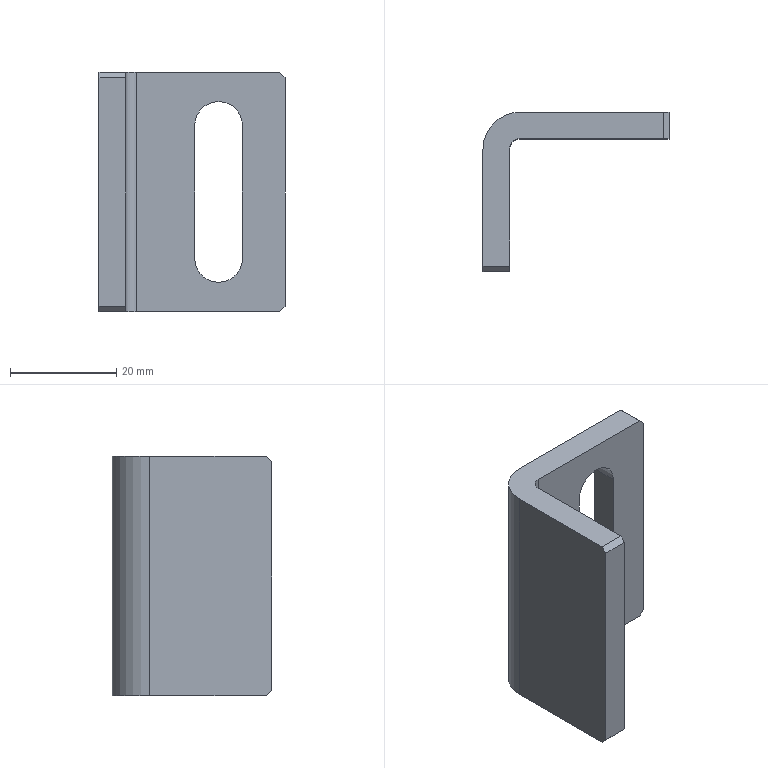Part | SolidWorks | features Fillet 2, Chamfer 1, ExtruThin 1, ICE 1 | 1 solid | 19 faces | box 35 x 30 x 45 mm | volume 11612 mm3 | plane 14 | cylinder 5 | commonest cylinder face diameters 9 x3 4 x1 14 x1
STEP:
#1=CARTESIAN_POINT('',(22.5,30.,5.5));
#2=VERTEX_POINT('',#1);
#3=CARTESIAN_POINT('',(27.,30.,10.));
#4=VERTEX_POINT('',#3);
#5=CARTESIAN_POINT('',(22.5,30.,10.));
#6=DIRECTION('',(0.,-1.,0.));
#7=DIRECTION('',(0.,0.,-1.));
#8=AXIS2_PLACEMENT_3D('',#5,#6,#7);
#9=CIRCLE('',#8,4.5);
#10=EDGE_CURVE('',#2,#4,#9,.T.);
#11=ORIENTED_EDGE('',*,*,#10,.F.);
#12=CARTESIAN_POINT('',(22.5,25.,5.5));
#13=VERTEX_POINT('',#12);
#14=CARTESIAN_POINT('',(22.5,30.,5.5));
#15=DIRECTION('',(0.,-1.,0.));
#16=VECTOR('',#15,1000.);
#17=LINE('',#14,#16);
#18=EDGE_CURVE('',#2,#13,#17,.T.);
#19=ORIENTED_EDGE('',*,*,#18,.T.);
#20=CARTESIAN_POINT('',(27.,25.,10.));
#21=VERTEX_POINT('',#20);
#22=CARTESIAN_POINT('',(22.5,25.,10.));
#23=DIRECTION('',(0.,-1.,0.));
#24=DIRECTION('',(0.,0.,-1.));
#25=AXIS2_PLACEMENT_3D('',#22,#23,#24);
#26=CIRCLE('',#25,4.5);
#27=EDGE_CURVE('',#13,#21,#26,.T.);
#28=ORIENTED_EDGE('',*,*,#27,.T.);
#29=CARTESIAN_POINT('',(27.,30.,10.));
#30=DIRECTION('',(0.,-1.,0.));
#31=VECTOR('',#30,1000.);
#32=LINE('',#29,#31);
#33=EDGE_CURVE('',#4,#21,#32,.T.);
#34=ORIENTED_EDGE('',*,*,#33,.F.);
#35=EDGE_LOOP('',(#11,#19,#28,#34));
#36=FACE_OUTER_BOUND('',#35,.T.);
#37=CARTESIAN_POINT('',(22.5,30.,10.));
#38=DIRECTION('',(0.,-1.,0.));
#39=DIRECTION('',(0.,0.,-1.));
#40=AXIS2_PLACEMENT_3D('',#37,#38,#39);
#41=CYLINDRICAL_SURFACE('',#40,4.5);
#42=ADVANCED_FACE('',(#36),#41,.F.);
#43=CARTESIAN_POINT('',(18.,25.,35.));
#44=VERTEX_POINT('',#43);
#45=CARTESIAN_POINT('',(18.,25.,10.));
#46=VERTEX_POINT('',#45);
#47=CARTESIAN_POINT('',(18.,25.,35.));
#48=DIRECTION('',(0.,0.,-1.));
#49=VECTOR('',#48,1000.);
#50=LINE('',#47,#49);
#51=EDGE_CURVE('',#44,#46,#50,.T.);
#52=ORIENTED_EDGE('',*,*,#51,.F.);
#53=CARTESIAN_POINT('',(27.,25.,35.));
#54=VERTEX_POINT('',#53);
#55=CARTESIAN_POINT('',(22.5,25.,35.));
#56=DIRECTION('',(0.,-1.,0.));
#57=DIRECTION('',(0.,0.,-1.));
#58=AXIS2_PLACEMENT_3D('',#55,#56,#57);
#59=CIRCLE('',#58,4.5);
#60=EDGE_CURVE('',#54,#44,#59,.T.);
#61=ORIENTED_EDGE('',*,*,#60,.F.);
#62=CARTESIAN_POINT('',(27.,25.,35.));
#63=DIRECTION('',(0.,0.,1.));
#64=VECTOR('',#63,1000.);
#65=LINE('',#62,#64);
#66=EDGE_CURVE('',#21,#54,#65,.T.);
#67=ORIENTED_EDGE('',*,*,#66,.F.);
#68=ORIENTED_EDGE('',*,*,#27,.F.);
#69=CARTESIAN_POINT('',(22.5,25.,10.));
#70=DIRECTION('',(0.,-1.,0.));
#71=DIRECTION('',(0.,0.,-1.));
#72=AXIS2_PLACEMENT_3D('',#69,#70,#71);
#73=CIRCLE('',#72,4.5);
#74=EDGE_CURVE('',#46,#13,#73,.T.);
#75=ORIENTED_EDGE('',*,*,#74,.F.);
#76=EDGE_LOOP('',(#52,#61,#67,#68,#75));
#77=FACE_BOUND('',#76,.T.);
#78=CARTESIAN_POINT('',(7.,25.,0.));
#79=VERTEX_POINT('',#78);
#80=CARTESIAN_POINT('',(34.,25.,0.));
#81=VERTEX_POINT('',#80);
#82=CARTESIAN_POINT('',(0.,25.,0.));
#83=DIRECTION('',(1.,0.,0.));
#84=VECTOR('',#83,1000.);
#85=LINE('',#82,#84);
#86=EDGE_CURVE('',#79,#81,#85,.T.);
#87=ORIENTED_EDGE('',*,*,#86,.T.);
#88=CARTESIAN_POINT('',(35.,25.,1.));
#89=VERTEX_POINT('',#88);
#90=CARTESIAN_POINT('',(34.,25.,0.));
#91=DIRECTION('',(0.7071,0.,0.7071));
#92=VECTOR('',#91,1000.);
#93=LINE('',#90,#92);
#94=EDGE_CURVE('',#81,#89,#93,.T.);
#95=ORIENTED_EDGE('',*,*,#94,.T.);
#96=CARTESIAN_POINT('',(35.,25.,44.));
#97=VERTEX_POINT('',#96);
#98=CARTESIAN_POINT('',(35.,25.,45.));
#99=DIRECTION('',(0.,0.,-1.));
#100=VECTOR('',#99,1000.);
#101=LINE('',#98,#100);
#102=EDGE_CURVE('',#97,#89,#101,.T.);
#103=ORIENTED_EDGE('',*,*,#102,.F.);
#104=CARTESIAN_POINT('',(34.,25.,45.));
#105=VERTEX_POINT('',#104);
#106=CARTESIAN_POINT('',(35.,25.,44.));
#107=DIRECTION('',(-0.7071,0.,0.7071));
#108=VECTOR('',#107,1000.);
#109=LINE('',#106,#108);
#110=EDGE_CURVE('',#97,#105,#109,.T.);
#111=ORIENTED_EDGE('',*,*,#110,.T.);
#112=CARTESIAN_POINT('',(7.,25.,45.));
#113=VERTEX_POINT('',#112);
#114=CARTESIAN_POINT('',(0.,25.,45.));
#115=DIRECTION('',(1.,0.,0.));
#116=VECTOR('',#115,1000.);
#117=LINE('',#114,#116);
#118=EDGE_CURVE('',#113,#105,#117,.T.);
#119=ORIENTED_EDGE('',*,*,#118,.F.);
#120=CARTESIAN_POINT('',(7.,25.,0.));
#121=DIRECTION('',(0.,0.,-1.));
#122=VECTOR('',#121,1000.);
#123=LINE('',#120,#122);
#124=EDGE_CURVE('',#113,#79,#123,.T.);
#125=ORIENTED_EDGE('',*,*,#124,.T.);
#126=EDGE_LOOP('',(#87,#95,#103,#111,#119,#125));
#127=FACE_OUTER_BOUND('',#126,.T.);
#128=CARTESIAN_POINT('',(0.,25.,45.));
#129=DIRECTION('',(0.,1.,0.));
#130=DIRECTION('',(0.,0.,1.));
#131=AXIS2_PLACEMENT_3D('',#128,#129,#130);
#132=PLANE('',#131);
#133=ADVANCED_FACE('',(#77,#127),#132,.F.);
#134=ORIENTED_EDGE('',*,*,#102,.T.);
#135=CARTESIAN_POINT('',(35.,30.,1.));
#136=VERTEX_POINT('',#135);
#137=CARTESIAN_POINT('',(35.,30.,1.));
#138=DIRECTION('',(0.,1.,0.));
#139=VECTOR('',#138,1000.);
#140=LINE('',#137,#139);
#141=EDGE_CURVE('',#89,#136,#140,.T.);
#142=ORIENTED_EDGE('',*,*,#141,.T.);
#143=CARTESIAN_POINT('',(35.,30.,44.));
#144=VERTEX_POINT('',#143);
#145=CARTESIAN_POINT('',(35.,30.,45.));
#146=DIRECTION('',(0.,0.,-1.));
#147=VECTOR('',#146,1000.);
#148=LINE('',#145,#147);
#149=EDGE_CURVE('',#144,#136,#148,.T.);
#150=ORIENTED_EDGE('',*,*,#149,.F.);
#151=CARTESIAN_POINT('',(35.,25.,44.));
#152=DIRECTION('',(0.,-1.,0.));
#153=VECTOR('',#152,1000.);
#154=LINE('',#151,#153);
#155=EDGE_CURVE('',#144,#97,#154,.T.);
#156=ORIENTED_EDGE('',*,*,#155,.T.);
#157=EDGE_LOOP('',(#134,#142,#150,#156));
#158=FACE_OUTER_BOUND('',#157,.T.);
#159=CARTESIAN_POINT('',(35.,30.,45.));
#160=DIRECTION('',(1.,0.,0.));
#161=DIRECTION('',(0.,0.,-1.));
#162=AXIS2_PLACEMENT_3D('',#159,#160,#161);
#163=PLANE('',#162);
#164=ADVANCED_FACE('',(#158),#163,.T.);
#165=CARTESIAN_POINT('',(27.,30.,35.));
#166=VERTEX_POINT('',#165);
#167=CARTESIAN_POINT('',(18.,30.,35.));
#168=VERTEX_POINT('',#167);
#169=CARTESIAN_POINT('',(22.5,30.,35.));
#170=DIRECTION('',(0.,-1.,0.));
#171=DIRECTION('',(0.,0.,-1.));
#172=AXIS2_PLACEMENT_3D('',#169,#170,#171);
#173=CIRCLE('',#172,4.5);
#174=EDGE_CURVE('',#166,#168,#173,.T.);
#175=ORIENTED_EDGE('',*,*,#174,.T.);
#176=CARTESIAN_POINT('',(18.,30.,10.));
#177=VERTEX_POINT('',#176);
#178=CARTESIAN_POINT('',(18.,30.,35.));
#179=DIRECTION('',(0.,0.,-1.));
#180=VECTOR('',#179,1000.);
#181=LINE('',#178,#180);
#182=EDGE_CURVE('',#168,#177,#181,.T.);
#183=ORIENTED_EDGE('',*,*,#182,.T.);
#184=CARTESIAN_POINT('',(22.5,30.,10.));
#185=DIRECTION('',(0.,-1.,0.));
#186=DIRECTION('',(0.,0.,-1.));
#187=AXIS2_PLACEMENT_3D('',#184,#185,#186);
#188=CIRCLE('',#187,4.5);
#189=EDGE_CURVE('',#177,#2,#188,.T.);
#190=ORIENTED_EDGE('',*,*,#189,.T.);
#191=ORIENTED_EDGE('',*,*,#10,.T.);
#192=CARTESIAN_POINT('',(27.,30.,35.));
#193=DIRECTION('',(0.,0.,1.));
#194=VECTOR('',#193,1000.);
#195=LINE('',#192,#194);
#196=EDGE_CURVE('',#4,#166,#195,.T.);
#197=ORIENTED_EDGE('',*,*,#196,.T.);
#198=EDGE_LOOP('',(#175,#183,#190,#191,#197));
#199=FACE_BOUND('',#198,.T.);
#200=ORIENTED_EDGE('',*,*,#149,.T.);
#201=CARTESIAN_POINT('',(34.,30.,0.));
#202=VERTEX_POINT('',#201);
#203=CARTESIAN_POINT('',(39.5,30.,5.5));
#204=DIRECTION('',(-0.7071,0.,-0.7071));
#205=VECTOR('',#204,1000.);
#206=LINE('',#203,#205);
#207=EDGE_CURVE('',#136,#202,#206,.T.);
#208=ORIENTED_EDGE('',*,*,#207,.T.);
#209=CARTESIAN_POINT('',(7.,30.,0.));
#210=VERTEX_POINT('',#209);
#211=CARTESIAN_POINT('',(0.,30.,0.));
#212=DIRECTION('',(1.,0.,0.));
#213=VECTOR('',#212,1000.);
#214=LINE('',#211,#213);
#215=EDGE_CURVE('',#210,#202,#214,.T.);
#216=ORIENTED_EDGE('',*,*,#215,.F.);
#217=CARTESIAN_POINT('',(7.,30.,45.));
#218=VERTEX_POINT('',#217);
#219=CARTESIAN_POINT('',(7.,30.,45.));
#220=DIRECTION('',(0.,0.,1.));
#221=VECTOR('',#220,1000.);
#222=LINE('',#219,#221);
#223=EDGE_CURVE('',#210,#218,#222,.T.);
#224=ORIENTED_EDGE('',*,*,#223,.T.);
#225=CARTESIAN_POINT('',(34.,30.,45.));
#226=VERTEX_POINT('',#225);
#227=CARTESIAN_POINT('',(0.,30.,45.));
#228=DIRECTION('',(1.,0.,0.));
#229=VECTOR('',#228,1000.);
#230=LINE('',#227,#229);
#231=EDGE_CURVE('',#218,#226,#230,.T.);
#232=ORIENTED_EDGE('',*,*,#231,.T.);
#233=CARTESIAN_POINT('',(17.,30.,62.));
#234=DIRECTION('',(0.7071,0.,-0.7071));
#235=VECTOR('',#234,1000.);
#236=LINE('',#233,#235);
#237=EDGE_CURVE('',#226,#144,#236,.T.);
#238=ORIENTED_EDGE('',*,*,#237,.T.);
#239=EDGE_LOOP('',(#200,#208,#216,#224,#232,#238));
#240=FACE_OUTER_BOUND('',#239,.T.);
#241=CARTESIAN_POINT('',(0.,30.,45.));
#242=DIRECTION('',(0.,1.,0.));
#243=DIRECTION('',(0.,0.,1.));
#244=AXIS2_PLACEMENT_3D('',#241,#242,#243);
#245=PLANE('',#244);
#246=ADVANCED_FACE('',(#199,#240),#245,.T.);
#247=CARTESIAN_POINT('',(0.,1.,0.));
#248=VERTEX_POINT('',#247);
#249=CARTESIAN_POINT('',(0.,23.,0.));
#250=VERTEX_POINT('',#249);
#251=CARTESIAN_POINT('',(0.,0.,0.));
#252=DIRECTION('',(0.,1.,0.));
#253=VECTOR('',#252,1000.);
#254=LINE('',#251,#253);
#255=EDGE_CURVE('',#248,#250,#254,.T.);
#256=ORIENTED_EDGE('',*,*,#255,.F.);
#257=CARTESIAN_POINT('',(0.,0.,1.));
#258=VERTEX_POINT('',#257);
#259=CARTESIAN_POINT('',(0.,-22.,23.));
#260=DIRECTION('',(0.,-0.7071,0.7071));
#261=VECTOR('',#260,1000.);
#262=LINE('',#259,#261);
#263=EDGE_CURVE('',#248,#258,#262,.T.);
#264=ORIENTED_EDGE('',*,*,#263,.T.);
#265=CARTESIAN_POINT('',(0.,0.,44.));
#266=VERTEX_POINT('',#265);
#267=CARTESIAN_POINT('',(0.,0.,45.));
#268=DIRECTION('',(0.,0.,-1.));
#269=VECTOR('',#268,1000.);
#270=LINE('',#267,#269);
#271=EDGE_CURVE('',#266,#258,#270,.T.);
#272=ORIENTED_EDGE('',*,*,#271,.F.);
#273=CARTESIAN_POINT('',(0.,1.,45.));
#274=VERTEX_POINT('',#273);
#275=CARTESIAN_POINT('',(0.,0.5,44.5));
#276=DIRECTION('',(0.,0.7071,0.7071));
#277=VECTOR('',#276,1000.);
#278=LINE('',#275,#277);
#279=EDGE_CURVE('',#266,#274,#278,.T.);
#280=ORIENTED_EDGE('',*,*,#279,.T.);
#281=CARTESIAN_POINT('',(0.,23.,45.));
#282=VERTEX_POINT('',#281);
#283=CARTESIAN_POINT('',(0.,0.,45.));
#284=DIRECTION('',(0.,1.,0.));
#285=VECTOR('',#284,1000.);
#286=LINE('',#283,#285);
#287=EDGE_CURVE('',#274,#282,#286,.T.);
#288=ORIENTED_EDGE('',*,*,#287,.T.);
#289=CARTESIAN_POINT('',(0.,23.,45.));
#290=DIRECTION('',(0.,0.,-1.));
#291=VECTOR('',#290,1000.);
#292=LINE('',#289,#291);
#293=EDGE_CURVE('',#282,#250,#292,.T.);
#294=ORIENTED_EDGE('',*,*,#293,.T.);
#295=EDGE_LOOP('',(#256,#264,#272,#280,#288,#294));
#296=FACE_OUTER_BOUND('',#295,.T.);
#297=CARTESIAN_POINT('',(0.,0.,45.));
#298=DIRECTION('',(-1.,0.,0.));
#299=DIRECTION('',(0.,0.,1.));
#300=AXIS2_PLACEMENT_3D('',#297,#298,#299);
#301=PLANE('',#300);
#302=ADVANCED_FACE('',(#296),#301,.T.);
#303=ORIENTED_EDGE('',*,*,#271,.T.);
#304=CARTESIAN_POINT('',(5.,0.,1.));
#305=VERTEX_POINT('',#304);
#306=CARTESIAN_POINT('',(5.,0.,1.));
#307=DIRECTION('',(1.,0.,0.));
#308=VECTOR('',#307,1000.);
#309=LINE('',#306,#308);
#310=EDGE_CURVE('',#258,#305,#309,.T.);
#311=ORIENTED_EDGE('',*,*,#310,.T.);
#312=CARTESIAN_POINT('',(5.,0.,44.));
#313=VERTEX_POINT('',#312);
#314=CARTESIAN_POINT('',(5.,0.,45.));
#315=DIRECTION('',(0.,0.,-1.));
#316=VECTOR('',#315,1000.);
#317=LINE('',#314,#316);
#318=EDGE_CURVE('',#313,#305,#317,.T.);
#319=ORIENTED_EDGE('',*,*,#318,.F.);
#320=CARTESIAN_POINT('',(0.,0.,44.));
#321=DIRECTION('',(-1.,0.,0.));
#322=VECTOR('',#321,1000.);
#323=LINE('',#320,#322);
#324=EDGE_CURVE('',#313,#266,#323,.T.);
#325=ORIENTED_EDGE('',*,*,#324,.T.);
#326=EDGE_LOOP('',(#303,#311,#319,#325));
#327=FACE_OUTER_BOUND('',#326,.T.);
#328=CARTESIAN_POINT('',(5.,0.,45.));
#329=DIRECTION('',(0.,-1.,0.));
#330=DIRECTION('',(0.,0.,-1.));
#331=AXIS2_PLACEMENT_3D('',#328,#329,#330);
#332=PLANE('',#331);
#333=ADVANCED_FACE('',(#327),#332,.T.);
#334=ORIENTED_EDGE('',*,*,#318,.T.);
#335=CARTESIAN_POINT('',(5.,1.,0.));
#336=VERTEX_POINT('',#335);
#337=CARTESIAN_POINT('',(5.,1.,0.));
#338=DIRECTION('',(0.,0.7071,-0.7071));
#339=VECTOR('',#338,1000.);
#340=LINE('',#337,#339);
#341=EDGE_CURVE('',#305,#336,#340,.T.);
#342=ORIENTED_EDGE('',*,*,#341,.T.);
#343=CARTESIAN_POINT('',(5.,23.,0.));
#344=VERTEX_POINT('',#343);
#345=CARTESIAN_POINT('',(5.,0.,0.));
#346=DIRECTION('',(0.,1.,0.));
#347=VECTOR('',#346,1000.);
#348=LINE('',#345,#347);
#349=EDGE_CURVE('',#336,#344,#348,.T.);
#350=ORIENTED_EDGE('',*,*,#349,.T.);
#351=CARTESIAN_POINT('',(5.,23.,45.));
#352=VERTEX_POINT('',#351);
#353=CARTESIAN_POINT('',(5.,23.,45.));
#354=DIRECTION('',(0.,0.,1.));
#355=VECTOR('',#354,1000.);
#356=LINE('',#353,#355);
#357=EDGE_CURVE('',#344,#352,#356,.T.);
#358=ORIENTED_EDGE('',*,*,#357,.T.);
#359=CARTESIAN_POINT('',(5.,1.,45.));
#360=VERTEX_POINT('',#359);
#361=CARTESIAN_POINT('',(5.,0.,45.));
#362=DIRECTION('',(0.,1.,0.));
#363=VECTOR('',#362,1000.);
#364=LINE('',#361,#363);
#365=EDGE_CURVE('',#360,#352,#364,.T.);
#366=ORIENTED_EDGE('',*,*,#365,.F.);
#367=CARTESIAN_POINT('',(5.,0.,44.));
#368=DIRECTION('',(0.,-0.7071,-0.7071));
#369=VECTOR('',#368,1000.);
#370=LINE('',#367,#369);
#371=EDGE_CURVE('',#360,#313,#370,.T.);
#372=ORIENTED_EDGE('',*,*,#371,.T.);
#373=EDGE_LOOP('',(#334,#342,#350,#358,#366,#372));
#374=FACE_OUTER_BOUND('',#373,.T.);
#375=CARTESIAN_POINT('',(5.,0.,45.));
#376=DIRECTION('',(-1.,0.,0.));
#377=DIRECTION('',(0.,0.,1.));
#378=AXIS2_PLACEMENT_3D('',#375,#376,#377);
#379=PLANE('',#378);
#380=ADVANCED_FACE('',(#374),#379,.F.);
#381=ORIENTED_EDGE('',*,*,#287,.F.);
#382=CARTESIAN_POINT('',(5.,1.,45.));
#383=DIRECTION('',(1.,0.,0.));
#384=VECTOR('',#383,1000.);
#385=LINE('',#382,#384);
#386=EDGE_CURVE('',#274,#360,#385,.T.);
#387=ORIENTED_EDGE('',*,*,#386,.T.);
#388=ORIENTED_EDGE('',*,*,#365,.T.);
#389=CARTESIAN_POINT('',(7.,23.,45.));
#390=DIRECTION('',(0.,0.,-1.));
#391=DIRECTION('',(-1.,0.,0.));
#392=AXIS2_PLACEMENT_3D('',#389,#390,#391);
#393=CIRCLE('',#392,2.);
#394=EDGE_CURVE('',#352,#113,#393,.T.);
#395=ORIENTED_EDGE('',*,*,#394,.T.);
#396=ORIENTED_EDGE('',*,*,#118,.T.);
#397=CARTESIAN_POINT('',(34.,30.,45.));
#398=DIRECTION('',(0.,1.,0.));
#399=VECTOR('',#398,1000.);
#400=LINE('',#397,#399);
#401=EDGE_CURVE('',#105,#226,#400,.T.);
#402=ORIENTED_EDGE('',*,*,#401,.T.);
#403=ORIENTED_EDGE('',*,*,#231,.F.);
#404=CARTESIAN_POINT('',(7.,23.,45.));
#405=DIRECTION('',(0.,0.,1.));
#406=DIRECTION('',(-1.,0.,0.));
#407=AXIS2_PLACEMENT_3D('',#404,#405,#406);
#408=CIRCLE('',#407,7.);
#409=EDGE_CURVE('',#218,#282,#408,.T.);
#410=ORIENTED_EDGE('',*,*,#409,.T.);
#411=EDGE_LOOP('',(#381,#387,#388,#395,#396,#402,#403,#410));
#412=FACE_OUTER_BOUND('',#411,.T.);
#413=CARTESIAN_POINT('',(0.,0.,45.));
#414=DIRECTION('',(0.,0.,-1.));
#415=DIRECTION('',(-1.,0.,0.));
#416=AXIS2_PLACEMENT_3D('',#413,#414,#415);
#417=PLANE('',#416);
#418=ADVANCED_FACE('',(#412),#417,.F.);
#419=ORIENTED_EDGE('',*,*,#349,.F.);
#420=CARTESIAN_POINT('',(0.,1.,0.));
#421=DIRECTION('',(-1.,0.,0.));
#422=VECTOR('',#421,1000.);
#423=LINE('',#420,#422);
#424=EDGE_CURVE('',#336,#248,#423,.T.);
#425=ORIENTED_EDGE('',*,*,#424,.T.);
#426=ORIENTED_EDGE('',*,*,#255,.T.);
#427=CARTESIAN_POINT('',(7.,23.,0.));
#428=DIRECTION('',(0.,0.,-1.));
#429=DIRECTION('',(-1.,0.,0.));
#430=AXIS2_PLACEMENT_3D('',#427,#428,#429);
#431=CIRCLE('',#430,7.);
#432=EDGE_CURVE('',#250,#210,#431,.T.);
#433=ORIENTED_EDGE('',*,*,#432,.T.);
#434=ORIENTED_EDGE('',*,*,#215,.T.);
#435=CARTESIAN_POINT('',(34.,0.,0.));
#436=DIRECTION('',(0.,-1.,0.));
#437=VECTOR('',#436,1000.);
#438=LINE('',#435,#437);
#439=EDGE_CURVE('',#202,#81,#438,.T.);
#440=ORIENTED_EDGE('',*,*,#439,.T.);
#441=ORIENTED_EDGE('',*,*,#86,.F.);
#442=CARTESIAN_POINT('',(7.,23.,0.));
#443=DIRECTION('',(0.,0.,1.));
#444=DIRECTION('',(-1.,0.,0.));
#445=AXIS2_PLACEMENT_3D('',#442,#443,#444);
#446=CIRCLE('',#445,2.);
#447=EDGE_CURVE('',#79,#344,#446,.T.);
#448=ORIENTED_EDGE('',*,*,#447,.T.);
#449=EDGE_LOOP('',(#419,#425,#426,#433,#434,#440,#441,#448));
#450=FACE_OUTER_BOUND('',#449,.T.);
#451=CARTESIAN_POINT('',(0.,0.,0.));
#452=DIRECTION('',(0.,0.,-1.));
#453=DIRECTION('',(-1.,0.,0.));
#454=AXIS2_PLACEMENT_3D('',#451,#452,#453);
#455=PLANE('',#454);
#456=ADVANCED_FACE('',(#450),#455,.T.);
#457=ORIENTED_EDGE('',*,*,#60,.T.);
#458=CARTESIAN_POINT('',(18.,30.,35.));
#459=DIRECTION('',(0.,-1.,0.));
#460=VECTOR('',#459,1000.);
#461=LINE('',#458,#460);
#462=EDGE_CURVE('',#168,#44,#461,.T.);
#463=ORIENTED_EDGE('',*,*,#462,.F.);
#464=ORIENTED_EDGE('',*,*,#174,.F.);
#465=CARTESIAN_POINT('',(27.,30.,35.));
#466=DIRECTION('',(0.,-1.,0.));
#467=VECTOR('',#466,1000.);
#468=LINE('',#465,#467);
#469=EDGE_CURVE('',#166,#54,#468,.T.);
#470=ORIENTED_EDGE('',*,*,#469,.T.);
#471=EDGE_LOOP('',(#457,#463,#464,#470));
#472=FACE_OUTER_BOUND('',#471,.T.);
#473=CARTESIAN_POINT('',(22.5,30.,35.));
#474=DIRECTION('',(0.,-1.,0.));
#475=DIRECTION('',(0.,0.,-1.));
#476=AXIS2_PLACEMENT_3D('',#473,#474,#475);
#477=CYLINDRICAL_SURFACE('',#476,4.5);
#478=ADVANCED_FACE('',(#472),#477,.F.);
#479=ORIENTED_EDGE('',*,*,#66,.T.);
#480=ORIENTED_EDGE('',*,*,#469,.F.);
#481=ORIENTED_EDGE('',*,*,#196,.F.);
#482=ORIENTED_EDGE('',*,*,#33,.T.);
#483=EDGE_LOOP('',(#479,#480,#481,#482));
#484=FACE_OUTER_BOUND('',#483,.T.);
#485=CARTESIAN_POINT('',(27.,30.,35.));
#486=DIRECTION('',(1.,0.,0.));
#487=DIRECTION('',(0.,0.,-1.));
#488=AXIS2_PLACEMENT_3D('',#485,#486,#487);
#489=PLANE('',#488);
#490=ADVANCED_FACE('',(#484),#489,.F.);
#491=ORIENTED_EDGE('',*,*,#18,.F.);
#492=ORIENTED_EDGE('',*,*,#189,.F.);
#493=CARTESIAN_POINT('',(18.,30.,10.));
#494=DIRECTION('',(0.,-1.,0.));
#495=VECTOR('',#494,1000.);
#496=LINE('',#493,#495);
#497=EDGE_CURVE('',#177,#46,#496,.T.);
#498=ORIENTED_EDGE('',*,*,#497,.T.);
#499=ORIENTED_EDGE('',*,*,#74,.T.);
#500=EDGE_LOOP('',(#491,#492,#498,#499));
#501=FACE_OUTER_BOUND('',#500,.T.);
#502=CARTESIAN_POINT('',(22.5,30.,10.));
#503=DIRECTION('',(0.,-1.,0.));
#504=DIRECTION('',(0.,0.,-1.));
#505=AXIS2_PLACEMENT_3D('',#502,#503,#504);
#506=CYLINDRICAL_SURFACE('',#505,4.5);
#507=ADVANCED_FACE('',(#501),#506,.F.);
#508=ORIENTED_EDGE('',*,*,#51,.T.);
#509=ORIENTED_EDGE('',*,*,#497,.F.);
#510=ORIENTED_EDGE('',*,*,#182,.F.);
#511=ORIENTED_EDGE('',*,*,#462,.T.);
#512=EDGE_LOOP('',(#508,#509,#510,#511));
#513=FACE_OUTER_BOUND('',#512,.T.);
#514=CARTESIAN_POINT('',(18.,30.,35.));
#515=DIRECTION('',(-1.,0.,0.));
#516=DIRECTION('',(0.,0.,1.));
#517=AXIS2_PLACEMENT_3D('',#514,#515,#516);
#518=PLANE('',#517);
#519=ADVANCED_FACE('',(#513),#518,.F.);
#520=ORIENTED_EDGE('',*,*,#394,.F.);
#521=ORIENTED_EDGE('',*,*,#357,.F.);
#522=ORIENTED_EDGE('',*,*,#447,.F.);
#523=ORIENTED_EDGE('',*,*,#124,.F.);
#524=EDGE_LOOP('',(#520,#521,#522,#523));
#525=FACE_OUTER_BOUND('',#524,.T.);
#526=CARTESIAN_POINT('',(7.,23.,45.));
#527=DIRECTION('',(0.,0.,1.));
#528=DIRECTION('',(1.,0.,0.));
#529=AXIS2_PLACEMENT_3D('',#526,#527,#528);
#530=CYLINDRICAL_SURFACE('',#529,2.);
#531=ADVANCED_FACE('',(#525),#530,.F.);
#532=ORIENTED_EDGE('',*,*,#409,.F.);
#533=ORIENTED_EDGE('',*,*,#223,.F.);
#534=ORIENTED_EDGE('',*,*,#432,.F.);
#535=ORIENTED_EDGE('',*,*,#293,.F.);
#536=EDGE_LOOP('',(#532,#533,#534,#535));
#537=FACE_OUTER_BOUND('',#536,.T.);
#538=CARTESIAN_POINT('',(7.,23.,45.));
#539=DIRECTION('',(0.,0.,-1.));
#540=DIRECTION('',(-1.,0.,0.));
#541=AXIS2_PLACEMENT_3D('',#538,#539,#540);
#542=CYLINDRICAL_SURFACE('',#541,7.);
#543=ADVANCED_FACE('',(#537),#542,.T.);
#544=ORIENTED_EDGE('',*,*,#341,.F.);
#545=ORIENTED_EDGE('',*,*,#310,.F.);
#546=ORIENTED_EDGE('',*,*,#263,.F.);
#547=ORIENTED_EDGE('',*,*,#424,.F.);
#548=EDGE_LOOP('',(#544,#545,#546,#547));
#549=FACE_OUTER_BOUND('',#548,.T.);
#550=CARTESIAN_POINT('',(0.,1.,0.));
#551=DIRECTION('',(0.,0.7071,0.7071));
#552=DIRECTION('',(-1.,0.,0.));
#553=AXIS2_PLACEMENT_3D('',#550,#551,#552);
#554=PLANE('',#553);
#555=ADVANCED_FACE('',(#549),#554,.F.);
#556=ORIENTED_EDGE('',*,*,#371,.F.);
#557=ORIENTED_EDGE('',*,*,#386,.F.);
#558=ORIENTED_EDGE('',*,*,#279,.F.);
#559=ORIENTED_EDGE('',*,*,#324,.F.);
#560=EDGE_LOOP('',(#556,#557,#558,#559));
#561=FACE_OUTER_BOUND('',#560,.T.);
#562=CARTESIAN_POINT('',(5.,0.,44.));
#563=DIRECTION('',(0.,-0.7071,0.7071));
#564=DIRECTION('',(1.,0.,0.));
#565=AXIS2_PLACEMENT_3D('',#562,#563,#564);
#566=PLANE('',#565);
#567=ADVANCED_FACE('',(#561),#566,.T.);
#568=ORIENTED_EDGE('',*,*,#207,.F.);
#569=ORIENTED_EDGE('',*,*,#141,.F.);
#570=ORIENTED_EDGE('',*,*,#94,.F.);
#571=ORIENTED_EDGE('',*,*,#439,.F.);
#572=EDGE_LOOP('',(#568,#569,#570,#571));
#573=FACE_OUTER_BOUND('',#572,.T.);
#574=CARTESIAN_POINT('',(34.,0.,0.));
#575=DIRECTION('',(-0.7071,0.,0.7071));
#576=DIRECTION('',(0.,-1.,0.));
#577=AXIS2_PLACEMENT_3D('',#574,#575,#576);
#578=PLANE('',#577);
#579=ADVANCED_FACE('',(#573),#578,.F.);
#580=ORIENTED_EDGE('',*,*,#237,.F.);
#581=ORIENTED_EDGE('',*,*,#401,.F.);
#582=ORIENTED_EDGE('',*,*,#110,.F.);
#583=ORIENTED_EDGE('',*,*,#155,.F.);
#584=EDGE_LOOP('',(#580,#581,#582,#583));
#585=FACE_OUTER_BOUND('',#584,.T.);
#586=CARTESIAN_POINT('',(35.,30.,44.));
#587=DIRECTION('',(0.7071,0.,0.7071));
#588=DIRECTION('',(0.,1.,0.));
#589=AXIS2_PLACEMENT_3D('',#586,#587,#588);
#590=PLANE('',#589);
#591=ADVANCED_FACE('',(#585),#590,.T.);
#592=CLOSED_SHELL('',(#42,#133,#164,#246,#302,#333,#380,#418,#456,#478,#490,#507,#519,#531,#543,#555,#567,#579,#591));
#593=MANIFOLD_SOLID_BREP('',#592);
#594=CARTESIAN_POINT('',(0.,0.,0.));
#595=DIRECTION('',(0.,0.,1.));
#596=DIRECTION('',(1.,0.,0.));
#597=AXIS2_PLACEMENT_3D('',#594,#595,#596);
#598=(LENGTH_UNIT()NAMED_UNIT(*)SI_UNIT(.MILLI.,.METRE.));
#599=UNCERTAINTY_MEASURE_WITH_UNIT(LENGTH_MEASURE(0.00001),#598,'','');
#600=(NAMED_UNIT(*)PLANE_ANGLE_UNIT()SI_UNIT($,.RADIAN.));
#601=(NAMED_UNIT(*)SI_UNIT($,.STERADIAN.)SOLID_ANGLE_UNIT());
#602=(GEOMETRIC_REPRESENTATION_CONTEXT(3)GLOBAL_UNCERTAINTY_ASSIGNED_CONTEXT((#599))GLOBAL_UNIT_ASSIGNED_CONTEXT((#598,#600,#601))REPRESENTATION_CONTEXT('',''));
#603=ADVANCED_BREP_SHAPE_REPRESENTATION('',(#593,#597),#602);